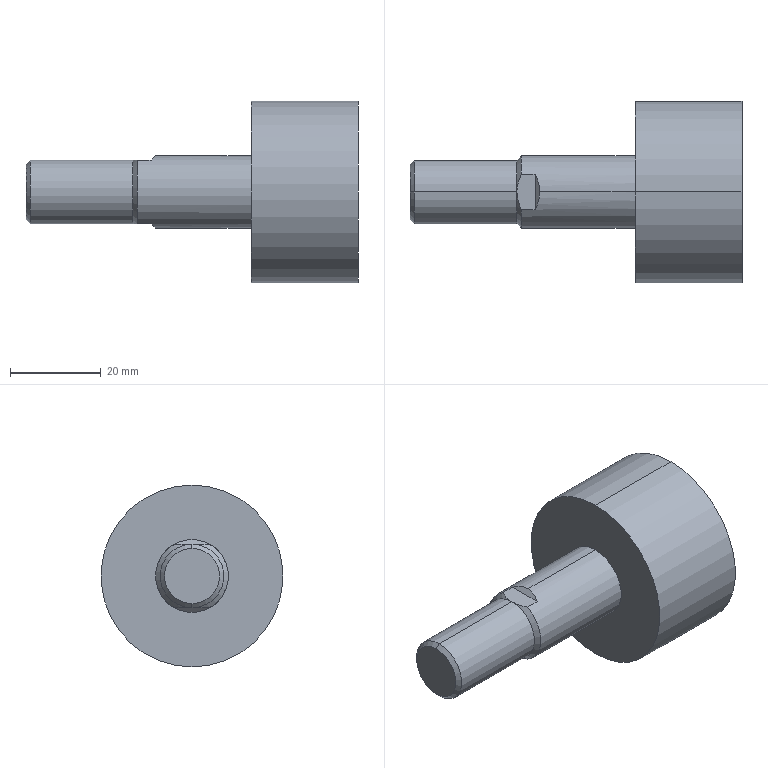Part | STEP file | 001-009-_ACQS-40x10-B_10r | 1 solid | 17 faces | box 73 x 40 x 40 mm | volume 38295 mm3 | plane 7 | cylinder 6 | cone 4 | commonest cylinder face diameters 14 x2 16 x2 40 x2